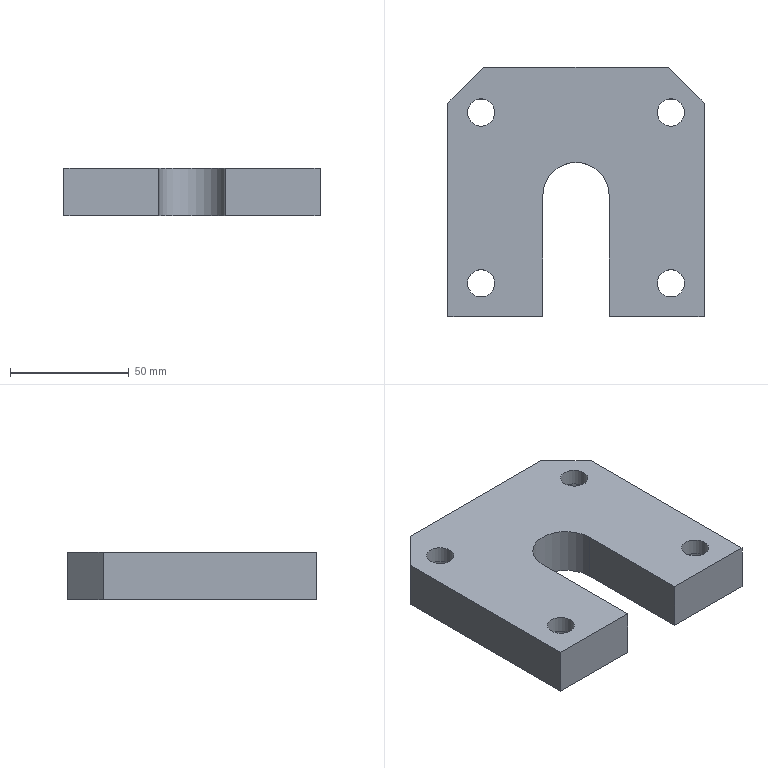Part | NX | features solid 2 | 1 solid | 24 faces | box 108 x 105 x 20 mm | volume 171442 mm3 | plane 15 | cylinder 9 | commonest cylinder face diameters 11.5 x4 18 x4 28 x1
STEP:
#1=CARTESIAN_POINT('',(2501.,-783.5,236.5));
#2=VERTEX_POINT('',#1);
#3=CARTESIAN_POINT('',(2510.,-783.5,236.5));
#4=DIRECTION('',(0.,0.,1.));
#5=DIRECTION('',(-1.,0.,0.));
#6=AXIS2_PLACEMENT_3D('',#3,#4,#5);
#7=CIRCLE('',#6,9.);
#8=EDGE_CURVE('',#2,#2,#7,.T.);
#9=ORIENTED_EDGE('',*,*,#8,.T.);
#10=EDGE_LOOP('',(#9));
#11=FACE_BOUND('',#10,.T.);
#12=CARTESIAN_POINT('',(2421.,-711.5,236.5));
#13=VERTEX_POINT('',#12);
#14=CARTESIAN_POINT('',(2430.,-711.5,236.5));
#15=DIRECTION('',(0.,0.,1.));
#16=DIRECTION('',(-1.,0.,0.));
#17=AXIS2_PLACEMENT_3D('',#14,#15,#16);
#18=CIRCLE('',#17,9.);
#19=EDGE_CURVE('',#13,#13,#18,.T.);
#20=ORIENTED_EDGE('',*,*,#19,.T.);
#21=EDGE_LOOP('',(#20));
#22=FACE_BOUND('',#21,.T.);
#23=CARTESIAN_POINT('',(2416.,-707.5,236.5));
#24=VERTEX_POINT('',#23);
#25=CARTESIAN_POINT('',(2416.,-797.5,236.5));
#26=VERTEX_POINT('',#25);
#27=CARTESIAN_POINT('',(2416.,-765.,236.5));
#28=DIRECTION('',(0.,-1.,0.));
#29=VECTOR('',#28,1000.);
#30=LINE('',#27,#29);
#31=EDGE_CURVE('',#24,#26,#30,.T.);
#32=ORIENTED_EDGE('',*,*,#31,.F.);
#33=CARTESIAN_POINT('',(2431.,-692.5,236.5));
#34=VERTEX_POINT('',#33);
#35=CARTESIAN_POINT('',(2414.25,-709.25,236.5));
#36=DIRECTION('',(0.7071,0.7071,0.));
#37=VECTOR('',#36,1000.);
#38=LINE('',#35,#37);
#39=EDGE_CURVE('',#24,#34,#38,.T.);
#40=ORIENTED_EDGE('',*,*,#39,.T.);
#41=CARTESIAN_POINT('',(2509.,-692.5,236.5));
#42=VERTEX_POINT('',#41);
#43=CARTESIAN_POINT('',(2470.,-692.5,236.5));
#44=DIRECTION('',(-1.,0.,0.));
#45=VECTOR('',#44,1000.);
#46=LINE('',#43,#45);
#47=EDGE_CURVE('',#42,#34,#46,.T.);
#48=ORIENTED_EDGE('',*,*,#47,.F.);
#49=CARTESIAN_POINT('',(2524.,-707.5,236.5));
#50=VERTEX_POINT('',#49);
#51=CARTESIAN_POINT('',(2525.75,-709.25,236.5));
#52=DIRECTION('',(0.7071,-0.7071,0.));
#53=VECTOR('',#52,1000.);
#54=LINE('',#51,#53);
#55=EDGE_CURVE('',#42,#50,#54,.T.);
#56=ORIENTED_EDGE('',*,*,#55,.T.);
#57=CARTESIAN_POINT('',(2524.,-797.5,236.5));
#58=VERTEX_POINT('',#57);
#59=CARTESIAN_POINT('',(2524.,-765.,236.5));
#60=DIRECTION('',(0.,1.,0.));
#61=VECTOR('',#60,1000.);
#62=LINE('',#59,#61);
#63=EDGE_CURVE('',#58,#50,#62,.T.);
#64=ORIENTED_EDGE('',*,*,#63,.F.);
#65=CARTESIAN_POINT('',(2484.,-797.5,236.5));
#66=VERTEX_POINT('',#65);
#67=CARTESIAN_POINT('',(2646.621,-797.5,236.5));
#68=DIRECTION('',(1.,0.,0.));
#69=VECTOR('',#68,1000.);
#70=LINE('',#67,#69);
#71=EDGE_CURVE('',#66,#58,#70,.T.);
#72=ORIENTED_EDGE('',*,*,#71,.F.);
#73=CARTESIAN_POINT('',(2484.,-746.5,236.5));
#74=VERTEX_POINT('',#73);
#75=CARTESIAN_POINT('',(2484.,-765.,236.5));
#76=DIRECTION('',(0.,1.,0.));
#77=VECTOR('',#76,1000.);
#78=LINE('',#75,#77);
#79=EDGE_CURVE('',#66,#74,#78,.T.);
#80=ORIENTED_EDGE('',*,*,#79,.T.);
#81=CARTESIAN_POINT('',(2456.,-746.5,236.5));
#82=VERTEX_POINT('',#81);
#83=CARTESIAN_POINT('',(2470.,-746.5,236.5));
#84=DIRECTION('',(0.,0.,-1.));
#85=DIRECTION('',(-1.,0.,0.));
#86=AXIS2_PLACEMENT_3D('',#83,#84,#85);
#87=CIRCLE('',#86,14.);
#88=EDGE_CURVE('',#82,#74,#87,.T.);
#89=ORIENTED_EDGE('',*,*,#88,.F.);
#90=CARTESIAN_POINT('',(2456.,-797.5,236.5));
#91=VERTEX_POINT('',#90);
#92=CARTESIAN_POINT('',(2456.,-765.,236.5));
#93=DIRECTION('',(0.,1.,0.));
#94=VECTOR('',#93,1000.);
#95=LINE('',#92,#94);
#96=EDGE_CURVE('',#91,#82,#95,.T.);
#97=ORIENTED_EDGE('',*,*,#96,.F.);
#98=CARTESIAN_POINT('',(2646.621,-797.5,236.5));
#99=DIRECTION('',(1.,0.,0.));
#100=VECTOR('',#99,1000.);
#101=LINE('',#98,#100);
#102=EDGE_CURVE('',#26,#91,#101,.T.);
#103=ORIENTED_EDGE('',*,*,#102,.F.);
#104=EDGE_LOOP('',(#32,#40,#48,#56,#64,#72,#80,#89,#97,#103));
#105=FACE_BOUND('',#104,.T.);
#106=CARTESIAN_POINT('',(2501.,-711.5,236.5));
#107=VERTEX_POINT('',#106);
#108=CARTESIAN_POINT('',(2510.,-711.5,236.5));
#109=DIRECTION('',(0.,0.,1.));
#110=DIRECTION('',(-1.,0.,0.));
#111=AXIS2_PLACEMENT_3D('',#108,#109,#110);
#112=CIRCLE('',#111,9.);
#113=EDGE_CURVE('',#107,#107,#112,.T.);
#114=ORIENTED_EDGE('',*,*,#113,.T.);
#115=EDGE_LOOP('',(#114));
#116=FACE_BOUND('',#115,.T.);
#117=CARTESIAN_POINT('',(2421.,-783.5,236.5));
#118=VERTEX_POINT('',#117);
#119=CARTESIAN_POINT('',(2430.,-783.5,236.5));
#120=DIRECTION('',(0.,0.,1.));
#121=DIRECTION('',(-1.,0.,0.));
#122=AXIS2_PLACEMENT_3D('',#119,#120,#121);
#123=CIRCLE('',#122,9.);
#124=EDGE_CURVE('',#118,#118,#123,.T.);
#125=ORIENTED_EDGE('',*,*,#124,.T.);
#126=EDGE_LOOP('',(#125));
#127=FACE_BOUND('',#126,.T.);
#128=CARTESIAN_POINT('',(2470.,-765.,236.5));
#129=DIRECTION('',(0.,0.,-1.));
#130=DIRECTION('',(1.,0.,0.));
#131=AXIS2_PLACEMENT_3D('',#128,#129,#130);
#132=PLANE('',#131);
#133=ADVANCED_FACE('',(#11,#22,#105,#116,#127),#132,.T.);
#134=CARTESIAN_POINT('',(2435.75,-783.5,256.5));
#135=VERTEX_POINT('',#134);
#136=CARTESIAN_POINT('',(2430.,-783.5,256.5));
#137=DIRECTION('',(0.,0.,1.));
#138=DIRECTION('',(1.,0.,0.));
#139=AXIS2_PLACEMENT_3D('',#136,#137,#138);
#140=CIRCLE('',#139,5.75);
#141=EDGE_CURVE('',#135,#135,#140,.T.);
#142=ORIENTED_EDGE('',*,*,#141,.F.);
#143=EDGE_LOOP('',(#142));
#144=FACE_BOUND('',#143,.T.);
#145=CARTESIAN_POINT('',(2515.75,-783.5,256.5));
#146=VERTEX_POINT('',#145);
#147=CARTESIAN_POINT('',(2510.,-783.5,256.5));
#148=DIRECTION('',(0.,0.,1.));
#149=DIRECTION('',(1.,0.,0.));
#150=AXIS2_PLACEMENT_3D('',#147,#148,#149);
#151=CIRCLE('',#150,5.75);
#152=EDGE_CURVE('',#146,#146,#151,.T.);
#153=ORIENTED_EDGE('',*,*,#152,.F.);
#154=EDGE_LOOP('',(#153));
#155=FACE_BOUND('',#154,.T.);
#156=CARTESIAN_POINT('',(2515.75,-711.5,256.5));
#157=VERTEX_POINT('',#156);
#158=CARTESIAN_POINT('',(2510.,-711.5,256.5));
#159=DIRECTION('',(0.,0.,1.));
#160=DIRECTION('',(1.,0.,0.));
#161=AXIS2_PLACEMENT_3D('',#158,#159,#160);
#162=CIRCLE('',#161,5.75);
#163=EDGE_CURVE('',#157,#157,#162,.T.);
#164=ORIENTED_EDGE('',*,*,#163,.F.);
#165=EDGE_LOOP('',(#164));
#166=FACE_BOUND('',#165,.T.);
#167=CARTESIAN_POINT('',(2435.75,-711.5,256.5));
#168=VERTEX_POINT('',#167);
#169=CARTESIAN_POINT('',(2430.,-711.5,256.5));
#170=DIRECTION('',(0.,0.,1.));
#171=DIRECTION('',(1.,0.,0.));
#172=AXIS2_PLACEMENT_3D('',#169,#170,#171);
#173=CIRCLE('',#172,5.75);
#174=EDGE_CURVE('',#168,#168,#173,.T.);
#175=ORIENTED_EDGE('',*,*,#174,.F.);
#176=EDGE_LOOP('',(#175));
#177=FACE_BOUND('',#176,.T.);
#178=CARTESIAN_POINT('',(2431.,-692.5,256.5));
#179=VERTEX_POINT('',#178);
#180=CARTESIAN_POINT('',(2509.,-692.5,256.5));
#181=VERTEX_POINT('',#180);
#182=CARTESIAN_POINT('',(2470.,-692.5,256.5));
#183=DIRECTION('',(1.,0.,0.));
#184=VECTOR('',#183,1000.);
#185=LINE('',#182,#184);
#186=EDGE_CURVE('',#179,#181,#185,.T.);
#187=ORIENTED_EDGE('',*,*,#186,.F.);
#188=CARTESIAN_POINT('',(2416.,-707.5,256.5));
#189=VERTEX_POINT('',#188);
#190=CARTESIAN_POINT('',(1934.25,-1189.25,256.5));
#191=DIRECTION('',(-0.7071,-0.7071,0.));
#192=VECTOR('',#191,1000.);
#193=LINE('',#190,#192);
#194=EDGE_CURVE('',#179,#189,#193,.T.);
#195=ORIENTED_EDGE('',*,*,#194,.T.);
#196=CARTESIAN_POINT('',(2416.,-797.5,256.5));
#197=VERTEX_POINT('',#196);
#198=CARTESIAN_POINT('',(2416.,-765.,256.5));
#199=DIRECTION('',(0.,1.,0.));
#200=VECTOR('',#199,1000.);
#201=LINE('',#198,#200);
#202=EDGE_CURVE('',#197,#189,#201,.T.);
#203=ORIENTED_EDGE('',*,*,#202,.F.);
#204=CARTESIAN_POINT('',(2456.,-797.5,256.5));
#205=VERTEX_POINT('',#204);
#206=CARTESIAN_POINT('',(2646.621,-797.5,256.5));
#207=DIRECTION('',(-1.,0.,0.));
#208=VECTOR('',#207,1000.);
#209=LINE('',#206,#208);
#210=EDGE_CURVE('',#205,#197,#209,.T.);
#211=ORIENTED_EDGE('',*,*,#210,.F.);
#212=CARTESIAN_POINT('',(2456.,-746.5,256.5));
#213=VERTEX_POINT('',#212);
#214=CARTESIAN_POINT('',(2456.,-746.5,256.5));
#215=DIRECTION('',(0.,-1.,0.));
#216=VECTOR('',#215,1000.);
#217=LINE('',#214,#216);
#218=EDGE_CURVE('',#213,#205,#217,.T.);
#219=ORIENTED_EDGE('',*,*,#218,.F.);
#220=CARTESIAN_POINT('',(2484.,-746.5,256.5));
#221=VERTEX_POINT('',#220);
#222=CARTESIAN_POINT('',(2470.,-746.5,256.5));
#223=DIRECTION('',(0.,0.,1.));
#224=DIRECTION('',(1.,0.,0.));
#225=AXIS2_PLACEMENT_3D('',#222,#223,#224);
#226=CIRCLE('',#225,14.);
#227=EDGE_CURVE('',#221,#213,#226,.T.);
#228=ORIENTED_EDGE('',*,*,#227,.F.);
#229=CARTESIAN_POINT('',(2484.,-797.5,256.5));
#230=VERTEX_POINT('',#229);
#231=CARTESIAN_POINT('',(2484.,0.,256.5));
#232=DIRECTION('',(0.,-1.,0.));
#233=VECTOR('',#232,1000.);
#234=LINE('',#231,#233);
#235=EDGE_CURVE('',#221,#230,#234,.T.);
#236=ORIENTED_EDGE('',*,*,#235,.T.);
#237=CARTESIAN_POINT('',(2524.,-797.5,256.5));
#238=VERTEX_POINT('',#237);
#239=CARTESIAN_POINT('',(2646.621,-797.5,256.5));
#240=DIRECTION('',(-1.,0.,0.));
#241=VECTOR('',#240,1000.);
#242=LINE('',#239,#241);
#243=EDGE_CURVE('',#238,#230,#242,.T.);
#244=ORIENTED_EDGE('',*,*,#243,.F.);
#245=CARTESIAN_POINT('',(2524.,-707.5,256.5));
#246=VERTEX_POINT('',#245);
#247=CARTESIAN_POINT('',(2524.,-765.,256.5));
#248=DIRECTION('',(0.,-1.,0.));
#249=VECTOR('',#248,1000.);
#250=LINE('',#247,#249);
#251=EDGE_CURVE('',#246,#238,#250,.T.);
#252=ORIENTED_EDGE('',*,*,#251,.F.);
#253=CARTESIAN_POINT('',(1280.75,535.75,256.5));
#254=DIRECTION('',(-0.7071,0.7071,0.));
#255=VECTOR('',#254,1000.);
#256=LINE('',#253,#255);
#257=EDGE_CURVE('',#246,#181,#256,.T.);
#258=ORIENTED_EDGE('',*,*,#257,.T.);
#259=EDGE_LOOP('',(#187,#195,#203,#211,#219,#228,#236,#244,#252,#258));
#260=FACE_BOUND('',#259,.T.);
#261=CARTESIAN_POINT('',(745.,0.,256.5));
#262=DIRECTION('',(0.,0.,1.));
#263=DIRECTION('',(-1.,0.,0.));
#264=AXIS2_PLACEMENT_3D('',#261,#262,#263);
#265=PLANE('',#264);
#266=ADVANCED_FACE('',(#144,#155,#166,#177,#260),#265,.T.);
#267=ORIENTED_EDGE('',*,*,#243,.T.);
#268=CARTESIAN_POINT('',(2484.,-797.5,1233.5));
#269=DIRECTION('',(0.,0.,1.));
#270=VECTOR('',#269,1000.);
#271=LINE('',#268,#270);
#272=EDGE_CURVE('',#66,#230,#271,.T.);
#273=ORIENTED_EDGE('',*,*,#272,.F.);
#274=ORIENTED_EDGE('',*,*,#71,.T.);
#275=CARTESIAN_POINT('',(2524.,-797.5,286.5));
#276=DIRECTION('',(0.,0.,-1.));
#277=VECTOR('',#276,1000.);
#278=LINE('',#275,#277);
#279=EDGE_CURVE('',#238,#58,#278,.T.);
#280=ORIENTED_EDGE('',*,*,#279,.F.);
#281=EDGE_LOOP('',(#267,#273,#274,#280));
#282=FACE_BOUND('',#281,.T.);
#283=CARTESIAN_POINT('',(2646.621,-797.5,-68.5));
#284=DIRECTION('',(0.,1.,0.));
#285=DIRECTION('',(-1.,0.,0.));
#286=AXIS2_PLACEMENT_3D('',#283,#284,#285);
#287=PLANE('',#286);
#288=ADVANCED_FACE('',(#282),#287,.F.);
#289=ORIENTED_EDGE('',*,*,#102,.T.);
#290=CARTESIAN_POINT('',(2456.,-797.5,1233.5));
#291=DIRECTION('',(0.,0.,-1.));
#292=VECTOR('',#291,1000.);
#293=LINE('',#290,#292);
#294=EDGE_CURVE('',#205,#91,#293,.T.);
#295=ORIENTED_EDGE('',*,*,#294,.F.);
#296=ORIENTED_EDGE('',*,*,#210,.T.);
#297=CARTESIAN_POINT('',(2416.,-797.5,-68.5));
#298=DIRECTION('',(0.,0.,-1.));
#299=VECTOR('',#298,1000.);
#300=LINE('',#297,#299);
#301=EDGE_CURVE('',#197,#26,#300,.T.);
#302=ORIENTED_EDGE('',*,*,#301,.T.);
#303=EDGE_LOOP('',(#289,#295,#296,#302));
#304=FACE_BOUND('',#303,.T.);
#305=CARTESIAN_POINT('',(2646.621,-797.5,-68.5));
#306=DIRECTION('',(0.,1.,0.));
#307=DIRECTION('',(-1.,0.,0.));
#308=AXIS2_PLACEMENT_3D('',#305,#306,#307);
#309=PLANE('',#308);
#310=ADVANCED_FACE('',(#304),#309,.F.);
#311=ORIENTED_EDGE('',*,*,#63,.T.);
#312=CARTESIAN_POINT('',(2524.,-707.5,286.5));
#313=DIRECTION('',(0.,0.,1.));
#314=VECTOR('',#313,1000.);
#315=LINE('',#312,#314);
#316=EDGE_CURVE('',#50,#246,#315,.T.);
#317=ORIENTED_EDGE('',*,*,#316,.T.);
#318=ORIENTED_EDGE('',*,*,#251,.T.);
#319=ORIENTED_EDGE('',*,*,#279,.T.);
#320=EDGE_LOOP('',(#311,#317,#318,#319));
#321=FACE_BOUND('',#320,.T.);
#322=CARTESIAN_POINT('',(2524.,-765.,286.5));
#323=DIRECTION('',(1.,0.,0.));
#324=DIRECTION('',(0.,0.,1.));
#325=AXIS2_PLACEMENT_3D('',#322,#323,#324);
#326=PLANE('',#325);
#327=ADVANCED_FACE('',(#321),#326,.T.);
#328=ORIENTED_EDGE('',*,*,#47,.T.);
#329=CARTESIAN_POINT('',(2431.,-692.5,286.5));
#330=DIRECTION('',(0.,0.,1.));
#331=VECTOR('',#330,1000.);
#332=LINE('',#329,#331);
#333=EDGE_CURVE('',#34,#179,#332,.T.);
#334=ORIENTED_EDGE('',*,*,#333,.T.);
#335=ORIENTED_EDGE('',*,*,#186,.T.);
#336=CARTESIAN_POINT('',(2509.,-692.5,286.5));
#337=DIRECTION('',(0.,0.,-1.));
#338=VECTOR('',#337,1000.);
#339=LINE('',#336,#338);
#340=EDGE_CURVE('',#181,#42,#339,.T.);
#341=ORIENTED_EDGE('',*,*,#340,.T.);
#342=EDGE_LOOP('',(#328,#334,#335,#341));
#343=FACE_BOUND('',#342,.T.);
#344=CARTESIAN_POINT('',(2470.,-692.5,286.5));
#345=DIRECTION('',(0.,1.,0.));
#346=DIRECTION('',(0.,0.,1.));
#347=AXIS2_PLACEMENT_3D('',#344,#345,#346);
#348=PLANE('',#347);
#349=ADVANCED_FACE('',(#343),#348,.T.);
#350=ORIENTED_EDGE('',*,*,#202,.T.);
#351=CARTESIAN_POINT('',(2416.,-707.5,286.5));
#352=DIRECTION('',(0.,0.,-1.));
#353=VECTOR('',#352,1000.);
#354=LINE('',#351,#353);
#355=EDGE_CURVE('',#189,#24,#354,.T.);
#356=ORIENTED_EDGE('',*,*,#355,.T.);
#357=ORIENTED_EDGE('',*,*,#31,.T.);
#358=ORIENTED_EDGE('',*,*,#301,.F.);
#359=EDGE_LOOP('',(#350,#356,#357,#358));
#360=FACE_BOUND('',#359,.T.);
#361=CARTESIAN_POINT('',(2416.,-765.,286.5));
#362=DIRECTION('',(-1.,0.,0.));
#363=DIRECTION('',(0.,0.,-1.));
#364=AXIS2_PLACEMENT_3D('',#361,#362,#363);
#365=PLANE('',#364);
#366=ADVANCED_FACE('',(#360),#365,.T.);
#367=ORIENTED_EDGE('',*,*,#235,.F.);
#368=CARTESIAN_POINT('',(2484.,-746.5,1233.5));
#369=DIRECTION('',(0.,0.,-1.));
#370=VECTOR('',#369,1000.);
#371=LINE('',#368,#370);
#372=EDGE_CURVE('',#221,#74,#371,.T.);
#373=ORIENTED_EDGE('',*,*,#372,.T.);
#374=ORIENTED_EDGE('',*,*,#79,.F.);
#375=ORIENTED_EDGE('',*,*,#272,.T.);
#376=EDGE_LOOP('',(#367,#373,#374,#375));
#377=FACE_BOUND('',#376,.T.);
#378=CARTESIAN_POINT('',(2484.,-797.5,1233.5));
#379=DIRECTION('',(-1.,0.,0.));
#380=DIRECTION('',(0.,0.,-1.));
#381=AXIS2_PLACEMENT_3D('',#378,#379,#380);
#382=PLANE('',#381);
#383=ADVANCED_FACE('',(#377),#382,.T.);
#384=ORIENTED_EDGE('',*,*,#227,.T.);
#385=CARTESIAN_POINT('',(2456.,-746.5,1233.5));
#386=DIRECTION('',(0.,0.,-1.));
#387=VECTOR('',#386,1000.);
#388=LINE('',#385,#387);
#389=EDGE_CURVE('',#213,#82,#388,.T.);
#390=ORIENTED_EDGE('',*,*,#389,.T.);
#391=ORIENTED_EDGE('',*,*,#88,.T.);
#392=ORIENTED_EDGE('',*,*,#372,.F.);
#393=EDGE_LOOP('',(#384,#390,#391,#392));
#394=FACE_BOUND('',#393,.T.);
#395=CARTESIAN_POINT('',(2470.,-746.5,1233.5));
#396=DIRECTION('',(0.,0.,-1.));
#397=DIRECTION('',(1.,0.,0.));
#398=AXIS2_PLACEMENT_3D('',#395,#396,#397);
#399=CYLINDRICAL_SURFACE('',#398,14.);
#400=ADVANCED_FACE('',(#394),#399,.F.);
#401=ORIENTED_EDGE('',*,*,#218,.T.);
#402=ORIENTED_EDGE('',*,*,#294,.T.);
#403=ORIENTED_EDGE('',*,*,#96,.T.);
#404=ORIENTED_EDGE('',*,*,#389,.F.);
#405=EDGE_LOOP('',(#401,#402,#403,#404));
#406=FACE_BOUND('',#405,.T.);
#407=CARTESIAN_POINT('',(2456.,-746.5,1233.5));
#408=DIRECTION('',(1.,0.,0.));
#409=DIRECTION('',(0.,0.,1.));
#410=AXIS2_PLACEMENT_3D('',#407,#408,#409);
#411=PLANE('',#410);
#412=ADVANCED_FACE('',(#406),#411,.T.);
#413=ORIENTED_EDGE('',*,*,#194,.F.);
#414=ORIENTED_EDGE('',*,*,#333,.F.);
#415=ORIENTED_EDGE('',*,*,#39,.F.);
#416=ORIENTED_EDGE('',*,*,#355,.F.);
#417=EDGE_LOOP('',(#413,#414,#415,#416));
#418=FACE_BOUND('',#417,.T.);
#419=CARTESIAN_POINT('',(2416.,-707.5,286.5));
#420=DIRECTION('',(0.7071,-0.7071,0.));
#421=DIRECTION('',(0.,0.,1.));
#422=AXIS2_PLACEMENT_3D('',#419,#420,#421);
#423=PLANE('',#422);
#424=ADVANCED_FACE('',(#418),#423,.F.);
#425=ORIENTED_EDGE('',*,*,#257,.F.);
#426=ORIENTED_EDGE('',*,*,#316,.F.);
#427=ORIENTED_EDGE('',*,*,#55,.F.);
#428=ORIENTED_EDGE('',*,*,#340,.F.);
#429=EDGE_LOOP('',(#425,#426,#427,#428));
#430=FACE_BOUND('',#429,.T.);
#431=CARTESIAN_POINT('',(2509.,-692.5,286.5));
#432=DIRECTION('',(-0.7071,-0.7071,0.));
#433=DIRECTION('',(0.,0.,1.));
#434=AXIS2_PLACEMENT_3D('',#431,#432,#433);
#435=PLANE('',#434);
#436=ADVANCED_FACE('',(#430),#435,.F.);
#437=ORIENTED_EDGE('',*,*,#174,.T.);
#438=EDGE_LOOP('',(#437));
#439=FACE_BOUND('',#438,.T.);
#440=CARTESIAN_POINT('',(2435.75,-711.5,249.5));
#441=VERTEX_POINT('',#440);
#442=CARTESIAN_POINT('',(2430.,-711.5,249.5));
#443=DIRECTION('',(0.,0.,1.));
#444=DIRECTION('',(1.,0.,0.));
#445=AXIS2_PLACEMENT_3D('',#442,#443,#444);
#446=CIRCLE('',#445,5.75);
#447=EDGE_CURVE('',#441,#441,#446,.T.);
#448=ORIENTED_EDGE('',*,*,#447,.F.);
#449=EDGE_LOOP('',(#448));
#450=FACE_BOUND('',#449,.T.);
#451=CARTESIAN_POINT('',(2430.,-711.5,234.5));
#452=DIRECTION('',(0.,0.,1.));
#453=DIRECTION('',(1.,0.,0.));
#454=AXIS2_PLACEMENT_3D('',#451,#452,#453);
#455=CYLINDRICAL_SURFACE('',#454,5.75);
#456=ADVANCED_FACE('',(#439,#450),#455,.F.);
#457=ORIENTED_EDGE('',*,*,#447,.T.);
#458=EDGE_LOOP('',(#457));
#459=FACE_BOUND('',#458,.T.);
#460=CARTESIAN_POINT('',(2421.,-711.5,249.5));
#461=VERTEX_POINT('',#460);
#462=CARTESIAN_POINT('',(2430.,-711.5,249.5));
#463=DIRECTION('',(0.,0.,1.));
#464=DIRECTION('',(-1.,0.,0.));
#465=AXIS2_PLACEMENT_3D('',#462,#463,#464);
#466=CIRCLE('',#465,9.);
#467=EDGE_CURVE('',#461,#461,#466,.T.);
#468=ORIENTED_EDGE('',*,*,#467,.F.);
#469=EDGE_LOOP('',(#468));
#470=FACE_BOUND('',#469,.T.);
#471=CARTESIAN_POINT('',(2430.,-711.5,249.5));
#472=DIRECTION('',(0.,0.,1.));
#473=DIRECTION('',(-1.,0.,0.));
#474=AXIS2_PLACEMENT_3D('',#471,#472,#473);
#475=PLANE('',#474);
#476=ADVANCED_FACE('',(#459,#470),#475,.F.);
#477=ORIENTED_EDGE('',*,*,#467,.T.);
#478=EDGE_LOOP('',(#477));
#479=FACE_BOUND('',#478,.T.);
#480=ORIENTED_EDGE('',*,*,#19,.F.);
#481=EDGE_LOOP('',(#480));
#482=FACE_BOUND('',#481,.T.);
#483=CARTESIAN_POINT('',(2430.,-711.5,236.5));
#484=DIRECTION('',(0.,0.,1.));
#485=DIRECTION('',(1.,0.,0.));
#486=AXIS2_PLACEMENT_3D('',#483,#484,#485);
#487=CYLINDRICAL_SURFACE('',#486,9.);
#488=ADVANCED_FACE('',(#479,#482),#487,.F.);
#489=ORIENTED_EDGE('',*,*,#163,.T.);
#490=EDGE_LOOP('',(#489));
#491=FACE_BOUND('',#490,.T.);
#492=CARTESIAN_POINT('',(2515.75,-711.5,249.5));
#493=VERTEX_POINT('',#492);
#494=CARTESIAN_POINT('',(2510.,-711.5,249.5));
#495=DIRECTION('',(0.,0.,1.));
#496=DIRECTION('',(1.,0.,0.));
#497=AXIS2_PLACEMENT_3D('',#494,#495,#496);
#498=CIRCLE('',#497,5.75);
#499=EDGE_CURVE('',#493,#493,#498,.T.);
#500=ORIENTED_EDGE('',*,*,#499,.F.);
#501=EDGE_LOOP('',(#500));
#502=FACE_BOUND('',#501,.T.);
#503=CARTESIAN_POINT('',(2510.,-711.5,234.5));
#504=DIRECTION('',(0.,0.,1.));
#505=DIRECTION('',(1.,0.,0.));
#506=AXIS2_PLACEMENT_3D('',#503,#504,#505);
#507=CYLINDRICAL_SURFACE('',#506,5.75);
#508=ADVANCED_FACE('',(#491,#502),#507,.F.);
#509=ORIENTED_EDGE('',*,*,#499,.T.);
#510=EDGE_LOOP('',(#509));
#511=FACE_BOUND('',#510,.T.);
#512=CARTESIAN_POINT('',(2501.,-711.5,249.5));
#513=VERTEX_POINT('',#512);
#514=CARTESIAN_POINT('',(2510.,-711.5,249.5));
#515=DIRECTION('',(0.,0.,1.));
#516=DIRECTION('',(-1.,0.,0.));
#517=AXIS2_PLACEMENT_3D('',#514,#515,#516);
#518=CIRCLE('',#517,9.);
#519=EDGE_CURVE('',#513,#513,#518,.T.);
#520=ORIENTED_EDGE('',*,*,#519,.F.);
#521=EDGE_LOOP('',(#520));
#522=FACE_BOUND('',#521,.T.);
#523=CARTESIAN_POINT('',(2510.,-711.5,249.5));
#524=DIRECTION('',(0.,0.,1.));
#525=DIRECTION('',(-1.,0.,0.));
#526=AXIS2_PLACEMENT_3D('',#523,#524,#525);
#527=PLANE('',#526);
#528=ADVANCED_FACE('',(#511,#522),#527,.F.);
#529=ORIENTED_EDGE('',*,*,#519,.T.);
#530=EDGE_LOOP('',(#529));
#531=FACE_BOUND('',#530,.T.);
#532=ORIENTED_EDGE('',*,*,#113,.F.);
#533=EDGE_LOOP('',(#532));
#534=FACE_BOUND('',#533,.T.);
#535=CARTESIAN_POINT('',(2510.,-711.5,236.5));
#536=DIRECTION('',(0.,0.,1.));
#537=DIRECTION('',(1.,0.,0.));
#538=AXIS2_PLACEMENT_3D('',#535,#536,#537);
#539=CYLINDRICAL_SURFACE('',#538,9.);
#540=ADVANCED_FACE('',(#531,#534),#539,.F.);
#541=ORIENTED_EDGE('',*,*,#152,.T.);
#542=EDGE_LOOP('',(#541));
#543=FACE_BOUND('',#542,.T.);
#544=CARTESIAN_POINT('',(2515.75,-783.5,249.5));
#545=VERTEX_POINT('',#544);
#546=CARTESIAN_POINT('',(2510.,-783.5,249.5));
#547=DIRECTION('',(0.,0.,1.));
#548=DIRECTION('',(1.,0.,0.));
#549=AXIS2_PLACEMENT_3D('',#546,#547,#548);
#550=CIRCLE('',#549,5.75);
#551=EDGE_CURVE('',#545,#545,#550,.T.);
#552=ORIENTED_EDGE('',*,*,#551,.F.);
#553=EDGE_LOOP('',(#552));
#554=FACE_BOUND('',#553,.T.);
#555=CARTESIAN_POINT('',(2510.,-783.5,234.5));
#556=DIRECTION('',(0.,0.,1.));
#557=DIRECTION('',(1.,0.,0.));
#558=AXIS2_PLACEMENT_3D('',#555,#556,#557);
#559=CYLINDRICAL_SURFACE('',#558,5.75);
#560=ADVANCED_FACE('',(#543,#554),#559,.F.);
#561=ORIENTED_EDGE('',*,*,#551,.T.);
#562=EDGE_LOOP('',(#561));
#563=FACE_BOUND('',#562,.T.);
#564=CARTESIAN_POINT('',(2501.,-783.5,249.5));
#565=VERTEX_POINT('',#564);
#566=CARTESIAN_POINT('',(2510.,-783.5,249.5));
#567=DIRECTION('',(0.,0.,1.));
#568=DIRECTION('',(-1.,0.,0.));
#569=AXIS2_PLACEMENT_3D('',#566,#567,#568);
#570=CIRCLE('',#569,9.);
#571=EDGE_CURVE('',#565,#565,#570,.T.);
#572=ORIENTED_EDGE('',*,*,#571,.F.);
#573=EDGE_LOOP('',(#572));
#574=FACE_BOUND('',#573,.T.);
#575=CARTESIAN_POINT('',(2510.,-783.5,249.5));
#576=DIRECTION('',(0.,0.,1.));
#577=DIRECTION('',(-1.,0.,0.));
#578=AXIS2_PLACEMENT_3D('',#575,#576,#577);
#579=PLANE('',#578);
#580=ADVANCED_FACE('',(#563,#574),#579,.F.);
#581=ORIENTED_EDGE('',*,*,#571,.T.);
#582=EDGE_LOOP('',(#581));
#583=FACE_BOUND('',#582,.T.);
#584=ORIENTED_EDGE('',*,*,#8,.F.);
#585=EDGE_LOOP('',(#584));
#586=FACE_BOUND('',#585,.T.);
#587=CARTESIAN_POINT('',(2510.,-783.5,236.5));
#588=DIRECTION('',(0.,0.,1.));
#589=DIRECTION('',(1.,0.,0.));
#590=AXIS2_PLACEMENT_3D('',#587,#588,#589);
#591=CYLINDRICAL_SURFACE('',#590,9.);
#592=ADVANCED_FACE('',(#583,#586),#591,.F.);
#593=ORIENTED_EDGE('',*,*,#141,.T.);
#594=EDGE_LOOP('',(#593));
#595=FACE_BOUND('',#594,.T.);
#596=CARTESIAN_POINT('',(2435.75,-783.5,249.5));
#597=VERTEX_POINT('',#596);
#598=CARTESIAN_POINT('',(2430.,-783.5,249.5));
#599=DIRECTION('',(0.,0.,1.));
#600=DIRECTION('',(1.,0.,0.));
#601=AXIS2_PLACEMENT_3D('',#598,#599,#600);
#602=CIRCLE('',#601,5.75);
#603=EDGE_CURVE('',#597,#597,#602,.T.);
#604=ORIENTED_EDGE('',*,*,#603,.F.);
#605=EDGE_LOOP('',(#604));
#606=FACE_BOUND('',#605,.T.);
#607=CARTESIAN_POINT('',(2430.,-783.5,234.5));
#608=DIRECTION('',(0.,0.,1.));
#609=DIRECTION('',(1.,0.,0.));
#610=AXIS2_PLACEMENT_3D('',#607,#608,#609);
#611=CYLINDRICAL_SURFACE('',#610,5.75);
#612=ADVANCED_FACE('',(#595,#606),#611,.F.);
#613=ORIENTED_EDGE('',*,*,#603,.T.);
#614=EDGE_LOOP('',(#613));
#615=FACE_BOUND('',#614,.T.);
#616=CARTESIAN_POINT('',(2421.,-783.5,249.5));
#617=VERTEX_POINT('',#616);
#618=CARTESIAN_POINT('',(2430.,-783.5,249.5));
#619=DIRECTION('',(0.,0.,1.));
#620=DIRECTION('',(-1.,0.,0.));
#621=AXIS2_PLACEMENT_3D('',#618,#619,#620);
#622=CIRCLE('',#621,9.);
#623=EDGE_CURVE('',#617,#617,#622,.T.);
#624=ORIENTED_EDGE('',*,*,#623,.F.);
#625=EDGE_LOOP('',(#624));
#626=FACE_BOUND('',#625,.T.);
#627=CARTESIAN_POINT('',(2430.,-783.5,249.5));
#628=DIRECTION('',(0.,0.,1.));
#629=DIRECTION('',(-1.,0.,0.));
#630=AXIS2_PLACEMENT_3D('',#627,#628,#629);
#631=PLANE('',#630);
#632=ADVANCED_FACE('',(#615,#626),#631,.F.);
#633=ORIENTED_EDGE('',*,*,#623,.T.);
#634=EDGE_LOOP('',(#633));
#635=FACE_BOUND('',#634,.T.);
#636=ORIENTED_EDGE('',*,*,#124,.F.);
#637=EDGE_LOOP('',(#636));
#638=FACE_BOUND('',#637,.T.);
#639=CARTESIAN_POINT('',(2430.,-783.5,236.5));
#640=DIRECTION('',(0.,0.,1.));
#641=DIRECTION('',(1.,0.,0.));
#642=AXIS2_PLACEMENT_3D('',#639,#640,#641);
#643=CYLINDRICAL_SURFACE('',#642,9.);
#644=ADVANCED_FACE('',(#635,#638),#643,.F.);
#645=CLOSED_SHELL('',(#133,#266,#288,#310,#327,#349,#366,#383,#400,#412,#424,#436,#456,#476,#488,#508,#528,#540,#560,#580,#592,#612,#632,#644));
#646=MANIFOLD_SOLID_BREP('',#645);
#647=(LENGTH_UNIT()NAMED_UNIT(*)SI_UNIT(.MILLI.,.METRE.));
#648=UNCERTAINTY_MEASURE_WITH_UNIT(LENGTH_MEASURE(0.00001),#647,'','');
#649=(NAMED_UNIT(*)PLANE_ANGLE_UNIT()SI_UNIT($,.RADIAN.));
#650=(NAMED_UNIT(*)SI_UNIT($,.STERADIAN.)SOLID_ANGLE_UNIT());
#651=(GEOMETRIC_REPRESENTATION_CONTEXT(3)GLOBAL_UNCERTAINTY_ASSIGNED_CONTEXT((#648))GLOBAL_UNIT_ASSIGNED_CONTEXT((#647,#649,#650))REPRESENTATION_CONTEXT('',''));
#652=ADVANCED_BREP_SHAPE_REPRESENTATION('',(#646),#651);